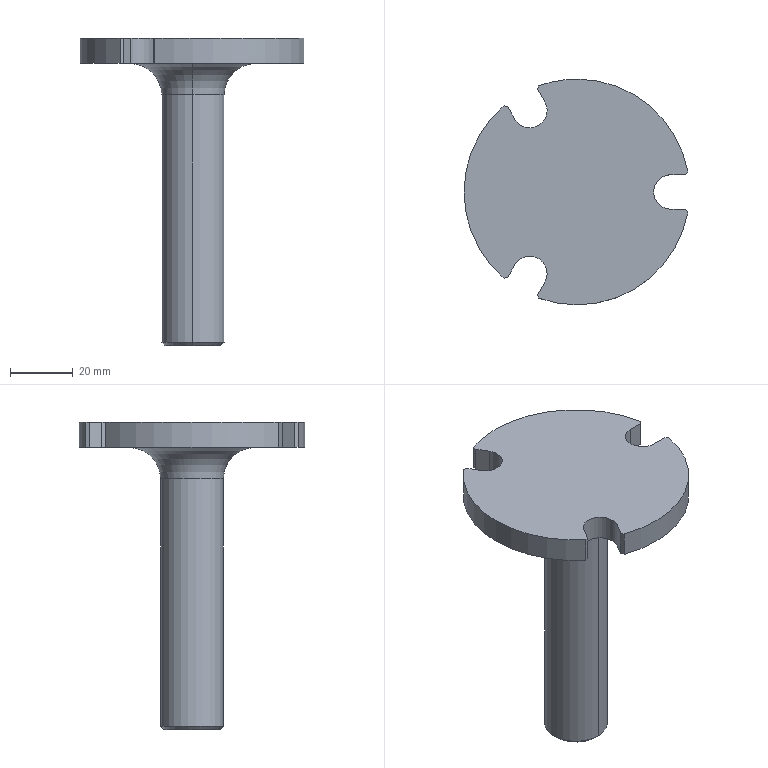Part | NX | 1 solid | 29 faces | box 71.434 x 72 x 98 mm | volume 59758 mm3 | plane 15 | cylinder 10 | torus 2 | cone 2 | commonest cylinder face diameters 11 x4 72 x4 20 x2
STEP:
#1=CARTESIAN_POINT('',(0.2829,20.,-8.));
#2=VERTEX_POINT('',#1);
#3=CARTESIAN_POINT('',(0.2829,-20.,-8.));
#4=VERTEX_POINT('',#3);
#5=CARTESIAN_POINT('',(0.2829,0.,-8.));
#6=DIRECTION('',(0.,0.,1.));
#7=DIRECTION('',(0.,-1.,0.));
#8=AXIS2_PLACEMENT_3D('',#5,#6,#7);
#9=CIRCLE('',#8,20.);
#10=EDGE_CURVE('',#2,#4,#9,.T.);
#11=ORIENTED_EDGE('',*,*,#10,.F.);
#12=CARTESIAN_POINT('',(0.2829,10.,-18.));
#13=VERTEX_POINT('',#12);
#14=CARTESIAN_POINT('',(0.2829,20.,-18.));
#15=DIRECTION('',(1.,0.,0.));
#16=DIRECTION('',(0.,1.,0.));
#17=AXIS2_PLACEMENT_3D('',#14,#15,#16);
#18=CIRCLE('',#17,10.);
#19=EDGE_CURVE('',#13,#2,#18,.F.);
#20=ORIENTED_EDGE('',*,*,#19,.F.);
#21=CARTESIAN_POINT('',(0.2829,-10.,-18.));
#22=VERTEX_POINT('',#21);
#23=CARTESIAN_POINT('',(0.2829,0.,-18.));
#24=DIRECTION('',(0.,0.,-1.));
#25=DIRECTION('',(0.,-1.,0.));
#26=AXIS2_PLACEMENT_3D('',#23,#24,#25);
#27=CIRCLE('',#26,10.);
#28=EDGE_CURVE('',#22,#13,#27,.T.);
#29=ORIENTED_EDGE('',*,*,#28,.F.);
#30=CARTESIAN_POINT('',(0.2829,-20.,-18.));
#31=DIRECTION('',(-1.,0.,0.));
#32=DIRECTION('',(0.,-1.,0.));
#33=AXIS2_PLACEMENT_3D('',#30,#31,#32);
#34=CIRCLE('',#33,10.);
#35=EDGE_CURVE('',#22,#4,#34,.F.);
#36=ORIENTED_EDGE('',*,*,#35,.T.);
#37=EDGE_LOOP('',(#11,#20,#29,#36));
#38=FACE_BOUND('',#37,.T.);
#39=CARTESIAN_POINT('',(0.2829,0.,-18.));
#40=DIRECTION('',(0.,0.,1.));
#41=DIRECTION('',(0.,1.,0.));
#42=AXIS2_PLACEMENT_3D('',#39,#40,#41);
#43=TOROIDAL_SURFACE('',#42,20.,10.);
#44=ADVANCED_FACE('',(#38),#43,.F.);
#45=CARTESIAN_POINT('',(-14.717,20.481,-8.));
#46=VERTEX_POINT('',#45);
#47=CARTESIAN_POINT('',(-9.954,28.731,-8.));
#48=VERTEX_POINT('',#47);
#49=CARTESIAN_POINT('',(-14.717,25.981,-8.));
#50=DIRECTION('',(0.,0.,1.));
#51=DIRECTION('',(0.866,0.5,0.));
#52=AXIS2_PLACEMENT_3D('',#49,#50,#51);
#53=CIRCLE('',#52,5.5);
#54=EDGE_CURVE('',#46,#48,#53,.T.);
#55=ORIENTED_EDGE('',*,*,#54,.F.);
#56=CARTESIAN_POINT('',(-14.717,20.481,0.));
#57=VERTEX_POINT('',#56);
#58=CARTESIAN_POINT('',(-14.717,20.481,-8.));
#59=DIRECTION('',(0.,0.,1.));
#60=VECTOR('',#59,1000.);
#61=LINE('',#58,#60);
#62=EDGE_CURVE('',#46,#57,#61,.T.);
#63=ORIENTED_EDGE('',*,*,#62,.T.);
#64=CARTESIAN_POINT('',(-9.954,28.731,0.));
#65=VERTEX_POINT('',#64);
#66=CARTESIAN_POINT('',(-14.717,25.981,0.));
#67=DIRECTION('',(0.,0.,1.));
#68=DIRECTION('',(0.866,0.5,0.));
#69=AXIS2_PLACEMENT_3D('',#66,#67,#68);
#70=CIRCLE('',#69,5.5);
#71=EDGE_CURVE('',#57,#65,#70,.T.);
#72=ORIENTED_EDGE('',*,*,#71,.T.);
#73=CARTESIAN_POINT('',(-9.954,28.731,-8.));
#74=DIRECTION('',(0.,0.,1.));
#75=VECTOR('',#74,1000.);
#76=LINE('',#73,#75);
#77=EDGE_CURVE('',#48,#65,#76,.T.);
#78=ORIENTED_EDGE('',*,*,#77,.F.);
#79=EDGE_LOOP('',(#55,#63,#72,#78));
#80=FACE_BOUND('',#79,.T.);
#81=CARTESIAN_POINT('',(-14.717,25.981,-8.));
#82=DIRECTION('',(0.,0.,1.));
#83=DIRECTION('',(0.,1.,0.));
#84=AXIS2_PLACEMENT_3D('',#81,#82,#83);
#85=CYLINDRICAL_SURFACE('',#84,5.5);
#86=ADVANCED_FACE('',(#80),#85,.F.);
#87=CARTESIAN_POINT('',(0.2829,36.,0.));
#88=VERTEX_POINT('',#87);
#89=CARTESIAN_POINT('',(-11.929,33.865,0.));
#90=VERTEX_POINT('',#89);
#91=CARTESIAN_POINT('',(0.2829,0.,0.));
#92=DIRECTION('',(0.,0.,1.));
#93=DIRECTION('',(0.,-1.,0.));
#94=AXIS2_PLACEMENT_3D('',#91,#92,#93);
#95=CIRCLE('',#94,36.);
#96=EDGE_CURVE('',#88,#90,#95,.T.);
#97=ORIENTED_EDGE('',*,*,#96,.F.);
#98=CARTESIAN_POINT('',(0.2829,36.,-8.));
#99=VERTEX_POINT('',#98);
#100=CARTESIAN_POINT('',(0.2829,36.,0.));
#101=DIRECTION('',(0.,0.,-1.));
#102=VECTOR('',#101,1000.);
#103=LINE('',#100,#102);
#104=EDGE_CURVE('',#88,#99,#103,.T.);
#105=ORIENTED_EDGE('',*,*,#104,.T.);
#106=CARTESIAN_POINT('',(-11.929,33.865,-8.));
#107=VERTEX_POINT('',#106);
#108=CARTESIAN_POINT('',(0.2829,0.,-8.));
#109=DIRECTION('',(0.,0.,1.));
#110=DIRECTION('',(0.,-1.,0.));
#111=AXIS2_PLACEMENT_3D('',#108,#109,#110);
#112=CIRCLE('',#111,36.);
#113=EDGE_CURVE('',#99,#107,#112,.T.);
#114=ORIENTED_EDGE('',*,*,#113,.T.);
#115=CARTESIAN_POINT('',(-11.929,33.865,0.));
#116=DIRECTION('',(0.,0.,1.));
#117=VECTOR('',#116,1000.);
#118=LINE('',#115,#117);
#119=EDGE_CURVE('',#107,#90,#118,.T.);
#120=ORIENTED_EDGE('',*,*,#119,.T.);
#121=EDGE_LOOP('',(#97,#105,#114,#120));
#122=FACE_BOUND('',#121,.T.);
#123=CARTESIAN_POINT('',(0.2829,0.,0.));
#124=DIRECTION('',(0.,0.,-1.));
#125=DIRECTION('',(0.,-1.,0.));
#126=AXIS2_PLACEMENT_3D('',#123,#124,#125);
#127=CYLINDRICAL_SURFACE('',#126,36.);
#128=ADVANCED_FACE('',(#122),#127,.T.);
#129=CARTESIAN_POINT('',(0.2829,9.,-98.));
#130=VERTEX_POINT('',#129);
#131=CARTESIAN_POINT('',(0.2829,-9.,-98.));
#132=VERTEX_POINT('',#131);
#133=CARTESIAN_POINT('',(0.2829,0.,-98.));
#134=DIRECTION('',(0.,0.,-1.));
#135=DIRECTION('',(0.,-1.,0.));
#136=AXIS2_PLACEMENT_3D('',#133,#134,#135);
#137=CIRCLE('',#136,9.);
#138=EDGE_CURVE('',#130,#132,#137,.T.);
#139=ORIENTED_EDGE('',*,*,#138,.F.);
#140=CARTESIAN_POINT('',(0.2829,10.,-97.));
#141=VERTEX_POINT('',#140);
#142=CARTESIAN_POINT('',(0.2829,10.,-97.));
#143=DIRECTION('',(0.,0.7071,0.7071));
#144=VECTOR('',#143,1000.);
#145=LINE('',#142,#144);
#146=EDGE_CURVE('',#141,#130,#145,.F.);
#147=ORIENTED_EDGE('',*,*,#146,.F.);
#148=CARTESIAN_POINT('',(0.2829,-10.,-97.));
#149=VERTEX_POINT('',#148);
#150=CARTESIAN_POINT('',(0.2829,0.,-97.));
#151=DIRECTION('',(0.,0.,1.));
#152=DIRECTION('',(0.,-1.,0.));
#153=AXIS2_PLACEMENT_3D('',#150,#151,#152);
#154=CIRCLE('',#153,10.);
#155=EDGE_CURVE('',#149,#141,#154,.T.);
#156=ORIENTED_EDGE('',*,*,#155,.F.);
#157=CARTESIAN_POINT('',(0.2829,-10.,-97.));
#158=DIRECTION('',(0.,-0.7071,0.7071));
#159=VECTOR('',#158,1000.);
#160=LINE('',#157,#159);
#161=EDGE_CURVE('',#149,#132,#160,.F.);
#162=ORIENTED_EDGE('',*,*,#161,.T.);
#163=EDGE_LOOP('',(#139,#147,#156,#162));
#164=FACE_BOUND('',#163,.T.);
#165=CARTESIAN_POINT('',(0.2829,0.,-97.));
#166=DIRECTION('',(0.,0.,1.));
#167=DIRECTION('',(0.,1.,0.));
#168=AXIS2_PLACEMENT_3D('',#165,#166,#167);
#169=CONICAL_SURFACE('',#168,10.,0.7854);
#170=ADVANCED_FACE('',(#164),#169,.T.);
#171=CARTESIAN_POINT('',(0.2829,0.,-18.));
#172=DIRECTION('',(0.,0.,-1.));
#173=DIRECTION('',(0.,-1.,0.));
#174=AXIS2_PLACEMENT_3D('',#171,#172,#173);
#175=CIRCLE('',#174,10.);
#176=EDGE_CURVE('',#13,#22,#175,.T.);
#177=ORIENTED_EDGE('',*,*,#176,.T.);
#178=CARTESIAN_POINT('',(0.2829,-10.,-8.));
#179=DIRECTION('',(0.,0.,-1.));
#180=VECTOR('',#179,1000.);
#181=LINE('',#178,#180);
#182=EDGE_CURVE('',#149,#22,#181,.F.);
#183=ORIENTED_EDGE('',*,*,#182,.F.);
#184=ORIENTED_EDGE('',*,*,#155,.T.);
#185=CARTESIAN_POINT('',(0.2829,10.,-8.));
#186=DIRECTION('',(0.,0.,-1.));
#187=VECTOR('',#186,1000.);
#188=LINE('',#185,#187);
#189=EDGE_CURVE('',#141,#13,#188,.F.);
#190=ORIENTED_EDGE('',*,*,#189,.T.);
#191=EDGE_LOOP('',(#177,#183,#184,#190));
#192=FACE_BOUND('',#191,.T.);
#193=CARTESIAN_POINT('',(0.2829,0.,-8.));
#194=DIRECTION('',(0.,0.,-1.));
#195=DIRECTION('',(0.,-1.,0.));
#196=AXIS2_PLACEMENT_3D('',#193,#194,#195);
#197=CYLINDRICAL_SURFACE('',#196,10.);
#198=ADVANCED_FACE('',(#192),#197,.T.);
#199=CARTESIAN_POINT('',(-11.929,-33.865,0.));
#200=VERTEX_POINT('',#199);
#201=CARTESIAN_POINT('',(35.717,-6.357,0.));
#202=VERTEX_POINT('',#201);
#203=CARTESIAN_POINT('',(0.2829,0.,0.));
#204=DIRECTION('',(0.,0.,1.));
#205=DIRECTION('',(0.,-1.,0.));
#206=AXIS2_PLACEMENT_3D('',#203,#204,#205);
#207=CIRCLE('',#206,36.);
#208=EDGE_CURVE('',#200,#202,#207,.T.);
#209=ORIENTED_EDGE('',*,*,#208,.F.);
#210=CARTESIAN_POINT('',(-11.929,-33.865,-8.));
#211=VERTEX_POINT('',#210);
#212=CARTESIAN_POINT('',(-11.929,-33.865,0.));
#213=DIRECTION('',(0.,0.,-1.));
#214=VECTOR('',#213,1000.);
#215=LINE('',#212,#214);
#216=EDGE_CURVE('',#200,#211,#215,.T.);
#217=ORIENTED_EDGE('',*,*,#216,.T.);
#218=CARTESIAN_POINT('',(35.717,-6.357,-8.));
#219=VERTEX_POINT('',#218);
#220=CARTESIAN_POINT('',(0.2829,0.,-8.));
#221=DIRECTION('',(0.,0.,1.));
#222=DIRECTION('',(0.,-1.,0.));
#223=AXIS2_PLACEMENT_3D('',#220,#221,#222);
#224=CIRCLE('',#223,36.);
#225=EDGE_CURVE('',#211,#219,#224,.T.);
#226=ORIENTED_EDGE('',*,*,#225,.T.);
#227=CARTESIAN_POINT('',(35.717,-6.357,0.));
#228=DIRECTION('',(0.,0.,1.));
#229=VECTOR('',#228,1000.);
#230=LINE('',#227,#229);
#231=EDGE_CURVE('',#219,#202,#230,.T.);
#232=ORIENTED_EDGE('',*,*,#231,.T.);
#233=EDGE_LOOP('',(#209,#217,#226,#232));
#234=FACE_BOUND('',#233,.T.);
#235=CARTESIAN_POINT('',(0.2829,0.,0.));
#236=DIRECTION('',(0.,0.,-1.));
#237=DIRECTION('',(0.,-1.,0.));
#238=AXIS2_PLACEMENT_3D('',#235,#236,#237);
#239=CYLINDRICAL_SURFACE('',#238,36.);
#240=ADVANCED_FACE('',(#234),#239,.T.);
#241=CARTESIAN_POINT('',(-22.94,27.509,0.));
#242=VERTEX_POINT('',#241);
#243=CARTESIAN_POINT('',(-22.94,-27.509,0.));
#244=VERTEX_POINT('',#243);
#245=CARTESIAN_POINT('',(0.2829,0.,0.));
#246=DIRECTION('',(0.,0.,1.));
#247=DIRECTION('',(0.,-1.,0.));
#248=AXIS2_PLACEMENT_3D('',#245,#246,#247);
#249=CIRCLE('',#248,36.);
#250=EDGE_CURVE('',#242,#244,#249,.T.);
#251=ORIENTED_EDGE('',*,*,#250,.F.);
#252=CARTESIAN_POINT('',(-22.94,27.509,-8.));
#253=VERTEX_POINT('',#252);
#254=CARTESIAN_POINT('',(-22.94,27.509,0.));
#255=DIRECTION('',(0.,0.,-1.));
#256=VECTOR('',#255,1000.);
#257=LINE('',#254,#256);
#258=EDGE_CURVE('',#242,#253,#257,.T.);
#259=ORIENTED_EDGE('',*,*,#258,.T.);
#260=CARTESIAN_POINT('',(-22.94,-27.509,-8.));
#261=VERTEX_POINT('',#260);
#262=CARTESIAN_POINT('',(0.2829,0.,-8.));
#263=DIRECTION('',(0.,0.,1.));
#264=DIRECTION('',(0.,-1.,0.));
#265=AXIS2_PLACEMENT_3D('',#262,#263,#264);
#266=CIRCLE('',#265,36.);
#267=EDGE_CURVE('',#253,#261,#266,.T.);
#268=ORIENTED_EDGE('',*,*,#267,.T.);
#269=CARTESIAN_POINT('',(-22.94,-27.509,0.));
#270=DIRECTION('',(0.,0.,1.));
#271=VECTOR('',#270,1000.);
#272=LINE('',#269,#271);
#273=EDGE_CURVE('',#261,#244,#272,.T.);
#274=ORIENTED_EDGE('',*,*,#273,.T.);
#275=EDGE_LOOP('',(#251,#259,#268,#274));
#276=FACE_BOUND('',#275,.T.);
#277=CARTESIAN_POINT('',(0.2829,0.,0.));
#278=DIRECTION('',(0.,0.,-1.));
#279=DIRECTION('',(0.,-1.,0.));
#280=AXIS2_PLACEMENT_3D('',#277,#278,#279);
#281=CYLINDRICAL_SURFACE('',#280,36.);
#282=ADVANCED_FACE('',(#276),#281,.T.);
#283=ORIENTED_EDGE('',*,*,#182,.T.);
#284=ORIENTED_EDGE('',*,*,#28,.T.);
#285=ORIENTED_EDGE('',*,*,#189,.F.);
#286=CARTESIAN_POINT('',(0.2829,0.,-97.));
#287=DIRECTION('',(0.,0.,1.));
#288=DIRECTION('',(0.,-1.,0.));
#289=AXIS2_PLACEMENT_3D('',#286,#287,#288);
#290=CIRCLE('',#289,10.);
#291=EDGE_CURVE('',#141,#149,#290,.T.);
#292=ORIENTED_EDGE('',*,*,#291,.T.);
#293=EDGE_LOOP('',(#283,#284,#285,#292));
#294=FACE_BOUND('',#293,.T.);
#295=CARTESIAN_POINT('',(0.2829,0.,-8.));
#296=DIRECTION('',(0.,0.,-1.));
#297=DIRECTION('',(0.,-1.,0.));
#298=AXIS2_PLACEMENT_3D('',#295,#296,#297);
#299=CYLINDRICAL_SURFACE('',#298,10.);
#300=ADVANCED_FACE('',(#294),#299,.T.);
#301=CARTESIAN_POINT('',(0.2829,0.,-98.));
#302=DIRECTION('',(0.,0.,-1.));
#303=DIRECTION('',(0.,-1.,0.));
#304=AXIS2_PLACEMENT_3D('',#301,#302,#303);
#305=CIRCLE('',#304,9.);
#306=EDGE_CURVE('',#132,#130,#305,.T.);
#307=ORIENTED_EDGE('',*,*,#306,.T.);
#308=ORIENTED_EDGE('',*,*,#138,.T.);
#309=EDGE_LOOP('',(#307,#308));
#310=FACE_BOUND('',#309,.T.);
#311=CARTESIAN_POINT('',(0.2829,0.,-98.));
#312=DIRECTION('',(0.,0.,1.));
#313=DIRECTION('',(0.,1.,0.));
#314=AXIS2_PLACEMENT_3D('',#311,#312,#313);
#315=PLANE('',#314);
#316=ADVANCED_FACE('',(#310),#315,.F.);
#317=ORIENTED_EDGE('',*,*,#146,.T.);
#318=ORIENTED_EDGE('',*,*,#306,.F.);
#319=ORIENTED_EDGE('',*,*,#161,.F.);
#320=ORIENTED_EDGE('',*,*,#291,.F.);
#321=EDGE_LOOP('',(#317,#318,#319,#320));
#322=FACE_BOUND('',#321,.T.);
#323=CARTESIAN_POINT('',(0.2829,0.,-97.));
#324=DIRECTION('',(0.,0.,1.));
#325=DIRECTION('',(0.,1.,0.));
#326=AXIS2_PLACEMENT_3D('',#323,#324,#325);
#327=CONICAL_SURFACE('',#326,10.,0.7854);
#328=ADVANCED_FACE('',(#322),#327,.T.);
#329=ORIENTED_EDGE('',*,*,#104,.F.);
#330=CARTESIAN_POINT('',(35.717,6.357,0.));
#331=VERTEX_POINT('',#330);
#332=CARTESIAN_POINT('',(0.2829,0.,0.));
#333=DIRECTION('',(0.,0.,1.));
#334=DIRECTION('',(0.,-1.,0.));
#335=AXIS2_PLACEMENT_3D('',#332,#333,#334);
#336=CIRCLE('',#335,36.);
#337=EDGE_CURVE('',#331,#88,#336,.T.);
#338=ORIENTED_EDGE('',*,*,#337,.F.);
#339=CARTESIAN_POINT('',(35.717,6.357,-8.));
#340=VERTEX_POINT('',#339);
#341=CARTESIAN_POINT('',(35.717,6.357,0.));
#342=DIRECTION('',(0.,0.,-1.));
#343=VECTOR('',#342,1000.);
#344=LINE('',#341,#343);
#345=EDGE_CURVE('',#331,#340,#344,.T.);
#346=ORIENTED_EDGE('',*,*,#345,.T.);
#347=CARTESIAN_POINT('',(0.2829,0.,-8.));
#348=DIRECTION('',(0.,0.,1.));
#349=DIRECTION('',(0.,-1.,0.));
#350=AXIS2_PLACEMENT_3D('',#347,#348,#349);
#351=CIRCLE('',#350,36.);
#352=EDGE_CURVE('',#340,#99,#351,.T.);
#353=ORIENTED_EDGE('',*,*,#352,.T.);
#354=EDGE_LOOP('',(#329,#338,#346,#353));
#355=FACE_BOUND('',#354,.T.);
#356=CARTESIAN_POINT('',(0.2829,0.,0.));
#357=DIRECTION('',(0.,0.,-1.));
#358=DIRECTION('',(0.,-1.,0.));
#359=AXIS2_PLACEMENT_3D('',#356,#357,#358);
#360=CYLINDRICAL_SURFACE('',#359,36.);
#361=ADVANCED_FACE('',(#355),#360,.T.);
#362=ORIENTED_EDGE('',*,*,#337,.T.);
#363=ORIENTED_EDGE('',*,*,#96,.T.);
#364=CARTESIAN_POINT('',(-12.243,32.695,0.));
#365=VERTEX_POINT('',#364);
#366=CARTESIAN_POINT('',(-19.577,5.322,0.));
#367=DIRECTION('',(-0.2588,-0.9659,0.));
#368=VECTOR('',#367,1000.);
#369=LINE('',#366,#368);
#370=EDGE_CURVE('',#90,#365,#369,.T.);
#371=ORIENTED_EDGE('',*,*,#370,.T.);
#372=CARTESIAN_POINT('',(-9.954,28.731,0.));
#373=DIRECTION('',(-0.5,0.866,0.));
#374=VECTOR('',#373,1000.);
#375=LINE('',#372,#374);
#376=EDGE_CURVE('',#65,#365,#375,.T.);
#377=ORIENTED_EDGE('',*,*,#376,.F.);
#378=ORIENTED_EDGE('',*,*,#71,.F.);
#379=CARTESIAN_POINT('',(-19.48,23.231,0.));
#380=VERTEX_POINT('',#379);
#381=CARTESIAN_POINT('',(-14.717,25.981,0.));
#382=DIRECTION('',(0.,0.,1.));
#383=DIRECTION('',(0.866,0.5,0.));
#384=AXIS2_PLACEMENT_3D('',#381,#382,#383);
#385=CIRCLE('',#384,5.5);
#386=EDGE_CURVE('',#380,#57,#385,.T.);
#387=ORIENTED_EDGE('',*,*,#386,.F.);
#388=CARTESIAN_POINT('',(-21.769,27.195,0.));
#389=VERTEX_POINT('',#388);
#390=CARTESIAN_POINT('',(-19.48,23.231,0.));
#391=DIRECTION('',(0.5,-0.866,0.));
#392=VECTOR('',#391,1000.);
#393=LINE('',#390,#392);
#394=EDGE_CURVE('',#389,#380,#393,.T.);
#395=ORIENTED_EDGE('',*,*,#394,.F.);
#396=CARTESIAN_POINT('',(5.604,19.86,0.));
#397=DIRECTION('',(-0.9659,0.2588,0.));
#398=VECTOR('',#397,1000.);
#399=LINE('',#396,#398);
#400=EDGE_CURVE('',#389,#242,#399,.T.);
#401=ORIENTED_EDGE('',*,*,#400,.T.);
#402=ORIENTED_EDGE('',*,*,#250,.T.);
#403=CARTESIAN_POINT('',(-21.769,-27.195,0.));
#404=VERTEX_POINT('',#403);
#405=CARTESIAN_POINT('',(5.604,-19.86,0.));
#406=DIRECTION('',(0.9659,0.2588,0.));
#407=VECTOR('',#406,1000.);
#408=LINE('',#405,#407);
#409=EDGE_CURVE('',#244,#404,#408,.T.);
#410=ORIENTED_EDGE('',*,*,#409,.T.);
#411=CARTESIAN_POINT('',(-19.48,-23.231,0.));
#412=VERTEX_POINT('',#411);
#413=CARTESIAN_POINT('',(-19.48,-23.231,0.));
#414=DIRECTION('',(-0.5,-0.866,0.));
#415=VECTOR('',#414,1000.);
#416=LINE('',#413,#415);
#417=EDGE_CURVE('',#412,#404,#416,.T.);
#418=ORIENTED_EDGE('',*,*,#417,.F.);
#419=CARTESIAN_POINT('',(-9.954,-28.731,0.));
#420=VERTEX_POINT('',#419);
#421=CARTESIAN_POINT('',(-14.717,-25.981,0.));
#422=DIRECTION('',(0.,0.,1.));
#423=DIRECTION('',(-0.866,0.5,0.));
#424=AXIS2_PLACEMENT_3D('',#421,#422,#423);
#425=CIRCLE('',#424,5.5);
#426=EDGE_CURVE('',#420,#412,#425,.T.);
#427=ORIENTED_EDGE('',*,*,#426,.F.);
#428=CARTESIAN_POINT('',(-12.243,-32.695,0.));
#429=VERTEX_POINT('',#428);
#430=CARTESIAN_POINT('',(-9.954,-28.731,0.));
#431=DIRECTION('',(0.5,0.866,0.));
#432=VECTOR('',#431,1000.);
#433=LINE('',#430,#432);
#434=EDGE_CURVE('',#429,#420,#433,.T.);
#435=ORIENTED_EDGE('',*,*,#434,.F.);
#436=CARTESIAN_POINT('',(-19.577,-5.322,0.));
#437=DIRECTION('',(0.2588,-0.9659,0.));
#438=VECTOR('',#437,1000.);
#439=LINE('',#436,#438);
#440=EDGE_CURVE('',#429,#200,#439,.T.);
#441=ORIENTED_EDGE('',*,*,#440,.T.);
#442=ORIENTED_EDGE('',*,*,#208,.T.);
#443=CARTESIAN_POINT('',(34.86,-5.5,0.));
#444=VERTEX_POINT('',#443);
#445=CARTESIAN_POINT('',(14.822,14.539,0.));
#446=DIRECTION('',(-0.7071,0.7071,0.));
#447=VECTOR('',#446,1000.);
#448=LINE('',#445,#447);
#449=EDGE_CURVE('',#202,#444,#448,.T.);
#450=ORIENTED_EDGE('',*,*,#449,.T.);
#451=CARTESIAN_POINT('',(30.283,-5.5,0.));
#452=VERTEX_POINT('',#451);
#453=CARTESIAN_POINT('',(30.283,-5.5,0.));
#454=DIRECTION('',(1.,0.,0.));
#455=VECTOR('',#454,1000.);
#456=LINE('',#453,#455);
#457=EDGE_CURVE('',#452,#444,#456,.T.);
#458=ORIENTED_EDGE('',*,*,#457,.F.);
#459=CARTESIAN_POINT('',(30.283,5.5,0.));
#460=VERTEX_POINT('',#459);
#461=CARTESIAN_POINT('',(30.283,0.,0.));
#462=DIRECTION('',(0.,0.,1.));
#463=DIRECTION('',(0.,-1.,0.));
#464=AXIS2_PLACEMENT_3D('',#461,#462,#463);
#465=CIRCLE('',#464,5.5);
#466=EDGE_CURVE('',#460,#452,#465,.T.);
#467=ORIENTED_EDGE('',*,*,#466,.F.);
#468=CARTESIAN_POINT('',(34.86,5.5,0.));
#469=VERTEX_POINT('',#468);
#470=CARTESIAN_POINT('',(30.283,5.5,0.));
#471=DIRECTION('',(-1.,0.,0.));
#472=VECTOR('',#471,1000.);
#473=LINE('',#470,#472);
#474=EDGE_CURVE('',#469,#460,#473,.T.);
#475=ORIENTED_EDGE('',*,*,#474,.F.);
#476=CARTESIAN_POINT('',(14.822,-14.539,0.));
#477=DIRECTION('',(0.7071,0.7071,0.));
#478=VECTOR('',#477,1000.);
#479=LINE('',#476,#478);
#480=EDGE_CURVE('',#469,#331,#479,.T.);
#481=ORIENTED_EDGE('',*,*,#480,.T.);
#482=EDGE_LOOP('',(#362,#363,#371,#377,#378,#387,#395,#401,#402,#410,#418,#427,#435,#441,#442,#450,#458,#467,#475,#481));
#483=FACE_BOUND('',#482,.T.);
#484=CARTESIAN_POINT('',(0.2829,0.,0.));
#485=DIRECTION('',(0.,0.,1.));
#486=DIRECTION('',(0.,1.,0.));
#487=AXIS2_PLACEMENT_3D('',#484,#485,#486);
#488=PLANE('',#487);
#489=ADVANCED_FACE('',(#483),#488,.T.);
#490=CARTESIAN_POINT('',(0.2829,0.,-8.));
#491=DIRECTION('',(0.,0.,1.));
#492=DIRECTION('',(0.,-1.,0.));
#493=AXIS2_PLACEMENT_3D('',#490,#491,#492);
#494=CIRCLE('',#493,20.);
#495=EDGE_CURVE('',#4,#2,#494,.T.);
#496=ORIENTED_EDGE('',*,*,#495,.T.);
#497=ORIENTED_EDGE('',*,*,#10,.T.);
#498=EDGE_LOOP('',(#496,#497));
#499=FACE_BOUND('',#498,.T.);
#500=CARTESIAN_POINT('',(-12.243,32.695,-8.));
#501=VERTEX_POINT('',#500);
#502=CARTESIAN_POINT('',(-9.954,28.731,-8.));
#503=DIRECTION('',(-0.5,0.866,0.));
#504=VECTOR('',#503,1000.);
#505=LINE('',#502,#504);
#506=EDGE_CURVE('',#48,#501,#505,.T.);
#507=ORIENTED_EDGE('',*,*,#506,.T.);
#508=CARTESIAN_POINT('',(-11.929,33.865,-8.));
#509=DIRECTION('',(0.2588,0.9659,0.));
#510=VECTOR('',#509,1000.);
#511=LINE('',#508,#510);
#512=EDGE_CURVE('',#501,#107,#511,.T.);
#513=ORIENTED_EDGE('',*,*,#512,.T.);
#514=ORIENTED_EDGE('',*,*,#113,.F.);
#515=ORIENTED_EDGE('',*,*,#352,.F.);
#516=CARTESIAN_POINT('',(34.86,5.5,-8.));
#517=VERTEX_POINT('',#516);
#518=CARTESIAN_POINT('',(35.717,6.357,-8.));
#519=DIRECTION('',(-0.7071,-0.7071,0.));
#520=VECTOR('',#519,1000.);
#521=LINE('',#518,#520);
#522=EDGE_CURVE('',#340,#517,#521,.T.);
#523=ORIENTED_EDGE('',*,*,#522,.T.);
#524=CARTESIAN_POINT('',(30.283,5.5,-8.));
#525=VERTEX_POINT('',#524);
#526=CARTESIAN_POINT('',(0.2829,5.5,-8.));
#527=DIRECTION('',(-1.,0.,0.));
#528=VECTOR('',#527,1000.);
#529=LINE('',#526,#528);
#530=EDGE_CURVE('',#517,#525,#529,.T.);
#531=ORIENTED_EDGE('',*,*,#530,.T.);
#532=CARTESIAN_POINT('',(30.283,-5.5,-8.));
#533=VERTEX_POINT('',#532);
#534=CARTESIAN_POINT('',(30.283,0.,-8.));
#535=DIRECTION('',(0.,0.,1.));
#536=DIRECTION('',(0.,-1.,0.));
#537=AXIS2_PLACEMENT_3D('',#534,#535,#536);
#538=CIRCLE('',#537,5.5);
#539=EDGE_CURVE('',#525,#533,#538,.T.);
#540=ORIENTED_EDGE('',*,*,#539,.T.);
#541=CARTESIAN_POINT('',(34.86,-5.5,-8.));
#542=VERTEX_POINT('',#541);
#543=CARTESIAN_POINT('',(30.283,-5.5,-8.));
#544=DIRECTION('',(1.,0.,0.));
#545=VECTOR('',#544,1000.);
#546=LINE('',#543,#545);
#547=EDGE_CURVE('',#533,#542,#546,.T.);
#548=ORIENTED_EDGE('',*,*,#547,.T.);
#549=CARTESIAN_POINT('',(35.717,-6.357,-8.));
#550=DIRECTION('',(0.7071,-0.7071,0.));
#551=VECTOR('',#550,1000.);
#552=LINE('',#549,#551);
#553=EDGE_CURVE('',#542,#219,#552,.T.);
#554=ORIENTED_EDGE('',*,*,#553,.T.);
#555=ORIENTED_EDGE('',*,*,#225,.F.);
#556=CARTESIAN_POINT('',(-12.243,-32.695,-8.));
#557=VERTEX_POINT('',#556);
#558=CARTESIAN_POINT('',(-11.929,-33.865,-8.));
#559=DIRECTION('',(-0.2588,0.9659,0.));
#560=VECTOR('',#559,1000.);
#561=LINE('',#558,#560);
#562=EDGE_CURVE('',#211,#557,#561,.T.);
#563=ORIENTED_EDGE('',*,*,#562,.T.);
#564=CARTESIAN_POINT('',(-9.954,-28.731,-8.));
#565=VERTEX_POINT('',#564);
#566=CARTESIAN_POINT('',(5.046,-2.75,-8.));
#567=DIRECTION('',(0.5,0.866,0.));
#568=VECTOR('',#567,1000.);
#569=LINE('',#566,#568);
#570=EDGE_CURVE('',#557,#565,#569,.T.);
#571=ORIENTED_EDGE('',*,*,#570,.T.);
#572=CARTESIAN_POINT('',(-19.48,-23.231,-8.));
#573=VERTEX_POINT('',#572);
#574=CARTESIAN_POINT('',(-14.717,-25.981,-8.));
#575=DIRECTION('',(0.,0.,1.));
#576=DIRECTION('',(-0.866,0.5,0.));
#577=AXIS2_PLACEMENT_3D('',#574,#575,#576);
#578=CIRCLE('',#577,5.5);
#579=EDGE_CURVE('',#565,#573,#578,.T.);
#580=ORIENTED_EDGE('',*,*,#579,.T.);
#581=CARTESIAN_POINT('',(-21.769,-27.195,-8.));
#582=VERTEX_POINT('',#581);
#583=CARTESIAN_POINT('',(-19.48,-23.231,-8.));
#584=DIRECTION('',(-0.5,-0.866,0.));
#585=VECTOR('',#584,1000.);
#586=LINE('',#583,#585);
#587=EDGE_CURVE('',#573,#582,#586,.T.);
#588=ORIENTED_EDGE('',*,*,#587,.T.);
#589=CARTESIAN_POINT('',(-22.94,-27.509,-8.));
#590=DIRECTION('',(-0.9659,-0.2588,0.));
#591=VECTOR('',#590,1000.);
#592=LINE('',#589,#591);
#593=EDGE_CURVE('',#582,#261,#592,.T.);
#594=ORIENTED_EDGE('',*,*,#593,.T.);
#595=ORIENTED_EDGE('',*,*,#267,.F.);
#596=CARTESIAN_POINT('',(-21.769,27.195,-8.));
#597=VERTEX_POINT('',#596);
#598=CARTESIAN_POINT('',(-22.94,27.509,-8.));
#599=DIRECTION('',(0.9659,-0.2588,0.));
#600=VECTOR('',#599,1000.);
#601=LINE('',#598,#600);
#602=EDGE_CURVE('',#253,#597,#601,.T.);
#603=ORIENTED_EDGE('',*,*,#602,.T.);
#604=CARTESIAN_POINT('',(-19.48,23.231,-8.));
#605=VERTEX_POINT('',#604);
#606=CARTESIAN_POINT('',(-4.48,-2.75,-8.));
#607=DIRECTION('',(0.5,-0.866,0.));
#608=VECTOR('',#607,1000.);
#609=LINE('',#606,#608);
#610=EDGE_CURVE('',#597,#605,#609,.T.);
#611=ORIENTED_EDGE('',*,*,#610,.T.);
#612=CARTESIAN_POINT('',(-14.717,25.981,-8.));
#613=DIRECTION('',(0.,0.,1.));
#614=DIRECTION('',(0.866,0.5,0.));
#615=AXIS2_PLACEMENT_3D('',#612,#613,#614);
#616=CIRCLE('',#615,5.5);
#617=EDGE_CURVE('',#605,#46,#616,.T.);
#618=ORIENTED_EDGE('',*,*,#617,.T.);
#619=ORIENTED_EDGE('',*,*,#54,.T.);
#620=EDGE_LOOP('',(#507,#513,#514,#515,#523,#531,#540,#548,#554,#555,#563,#571,#580,#588,#594,#595,#603,#611,#618,#619));
#621=FACE_BOUND('',#620,.T.);
#622=CARTESIAN_POINT('',(0.2829,0.,-8.));
#623=DIRECTION('',(0.,0.,1.));
#624=DIRECTION('',(0.,1.,0.));
#625=AXIS2_PLACEMENT_3D('',#622,#623,#624);
#626=PLANE('',#625);
#627=ADVANCED_FACE('',(#499,#621),#626,.F.);
#628=ORIENTED_EDGE('',*,*,#530,.F.);
#629=CARTESIAN_POINT('',(34.86,5.5,-8.));
#630=DIRECTION('',(0.,0.,1.));
#631=VECTOR('',#630,1000.);
#632=LINE('',#629,#631);
#633=EDGE_CURVE('',#517,#469,#632,.T.);
#634=ORIENTED_EDGE('',*,*,#633,.T.);
#635=ORIENTED_EDGE('',*,*,#474,.T.);
#636=CARTESIAN_POINT('',(30.283,5.5,-8.));
#637=DIRECTION('',(0.,0.,1.));
#638=VECTOR('',#637,1000.);
#639=LINE('',#636,#638);
#640=EDGE_CURVE('',#525,#460,#639,.T.);
#641=ORIENTED_EDGE('',*,*,#640,.F.);
#642=EDGE_LOOP('',(#628,#634,#635,#641));
#643=FACE_BOUND('',#642,.T.);
#644=CARTESIAN_POINT('',(30.283,5.5,-8.));
#645=DIRECTION('',(0.,1.,0.));
#646=DIRECTION('',(1.,0.,0.));
#647=AXIS2_PLACEMENT_3D('',#644,#645,#646);
#648=PLANE('',#647);
#649=ADVANCED_FACE('',(#643),#648,.F.);
#650=ORIENTED_EDGE('',*,*,#457,.T.);
#651=CARTESIAN_POINT('',(34.86,-5.5,-8.));
#652=DIRECTION('',(0.,0.,-1.));
#653=VECTOR('',#652,1000.);
#654=LINE('',#651,#653);
#655=EDGE_CURVE('',#444,#542,#654,.T.);
#656=ORIENTED_EDGE('',*,*,#655,.T.);
#657=ORIENTED_EDGE('',*,*,#547,.F.);
#658=CARTESIAN_POINT('',(30.283,-5.5,-8.));
#659=DIRECTION('',(0.,0.,1.));
#660=VECTOR('',#659,1000.);
#661=LINE('',#658,#660);
#662=EDGE_CURVE('',#533,#452,#661,.T.);
#663=ORIENTED_EDGE('',*,*,#662,.T.);
#664=EDGE_LOOP('',(#650,#656,#657,#663));
#665=FACE_BOUND('',#664,.T.);
#666=CARTESIAN_POINT('',(30.283,-5.5,-8.));
#667=DIRECTION('',(0.,-1.,0.));
#668=DIRECTION('',(-1.,0.,0.));
#669=AXIS2_PLACEMENT_3D('',#666,#667,#668);
#670=PLANE('',#669);
#671=ADVANCED_FACE('',(#665),#670,.F.);
#672=ORIENTED_EDGE('',*,*,#466,.T.);
#673=ORIENTED_EDGE('',*,*,#662,.F.);
#674=ORIENTED_EDGE('',*,*,#539,.F.);
#675=ORIENTED_EDGE('',*,*,#640,.T.);
#676=EDGE_LOOP('',(#672,#673,#674,#675));
#677=FACE_BOUND('',#676,.T.);
#678=CARTESIAN_POINT('',(30.283,0.,-8.));
#679=DIRECTION('',(0.,0.,1.));
#680=DIRECTION('',(0.,1.,0.));
#681=AXIS2_PLACEMENT_3D('',#678,#679,#680);
#682=CYLINDRICAL_SURFACE('',#681,5.5);
#683=ADVANCED_FACE('',(#677),#682,.F.);
#684=ORIENTED_EDGE('',*,*,#610,.F.);
#685=CARTESIAN_POINT('',(-21.769,27.195,-8.));
#686=DIRECTION('',(0.,0.,1.));
#687=VECTOR('',#686,1000.);
#688=LINE('',#685,#687);
#689=EDGE_CURVE('',#597,#389,#688,.T.);
#690=ORIENTED_EDGE('',*,*,#689,.T.);
#691=ORIENTED_EDGE('',*,*,#394,.T.);
#692=CARTESIAN_POINT('',(-19.48,23.231,-8.));
#693=DIRECTION('',(0.,0.,1.));
#694=VECTOR('',#693,1000.);
#695=LINE('',#692,#694);
#696=EDGE_CURVE('',#605,#380,#695,.T.);
#697=ORIENTED_EDGE('',*,*,#696,.F.);
#698=EDGE_LOOP('',(#684,#690,#691,#697));
#699=FACE_BOUND('',#698,.T.);
#700=CARTESIAN_POINT('',(-19.48,23.231,-8.));
#701=DIRECTION('',(-0.866,-0.5,0.));
#702=DIRECTION('',(-0.5,0.866,0.));
#703=AXIS2_PLACEMENT_3D('',#700,#701,#702);
#704=PLANE('',#703);
#705=ADVANCED_FACE('',(#699),#704,.F.);
#706=ORIENTED_EDGE('',*,*,#376,.T.);
#707=CARTESIAN_POINT('',(-12.243,32.695,-8.));
#708=DIRECTION('',(0.,0.,-1.));
#709=VECTOR('',#708,1000.);
#710=LINE('',#707,#709);
#711=EDGE_CURVE('',#365,#501,#710,.T.);
#712=ORIENTED_EDGE('',*,*,#711,.T.);
#713=ORIENTED_EDGE('',*,*,#506,.F.);
#714=ORIENTED_EDGE('',*,*,#77,.T.);
#715=EDGE_LOOP('',(#706,#712,#713,#714));
#716=FACE_BOUND('',#715,.T.);
#717=CARTESIAN_POINT('',(-9.954,28.731,-8.));
#718=DIRECTION('',(0.866,0.5,0.));
#719=DIRECTION('',(0.5,-0.866,0.));
#720=AXIS2_PLACEMENT_3D('',#717,#718,#719);
#721=PLANE('',#720);
#722=ADVANCED_FACE('',(#716),#721,.F.);
#723=ORIENTED_EDGE('',*,*,#62,.F.);
#724=ORIENTED_EDGE('',*,*,#617,.F.);
#725=ORIENTED_EDGE('',*,*,#696,.T.);
#726=ORIENTED_EDGE('',*,*,#386,.T.);
#727=EDGE_LOOP('',(#723,#724,#725,#726));
#728=FACE_BOUND('',#727,.T.);
#729=CARTESIAN_POINT('',(-14.717,25.981,-8.));
#730=DIRECTION('',(0.,0.,1.));
#731=DIRECTION('',(0.,1.,0.));
#732=AXIS2_PLACEMENT_3D('',#729,#730,#731);
#733=CYLINDRICAL_SURFACE('',#732,5.5);
#734=ADVANCED_FACE('',(#728),#733,.F.);
#735=ORIENTED_EDGE('',*,*,#570,.F.);
#736=CARTESIAN_POINT('',(-12.243,-32.695,-8.));
#737=DIRECTION('',(0.,0.,1.));
#738=VECTOR('',#737,1000.);
#739=LINE('',#736,#738);
#740=EDGE_CURVE('',#557,#429,#739,.T.);
#741=ORIENTED_EDGE('',*,*,#740,.T.);
#742=ORIENTED_EDGE('',*,*,#434,.T.);
#743=CARTESIAN_POINT('',(-9.954,-28.731,-8.));
#744=DIRECTION('',(0.,0.,1.));
#745=VECTOR('',#744,1000.);
#746=LINE('',#743,#745);
#747=EDGE_CURVE('',#565,#420,#746,.T.);
#748=ORIENTED_EDGE('',*,*,#747,.F.);
#749=EDGE_LOOP('',(#735,#741,#742,#748));
#750=FACE_BOUND('',#749,.T.);
#751=CARTESIAN_POINT('',(-9.954,-28.731,-8.));
#752=DIRECTION('',(0.866,-0.5,0.));
#753=DIRECTION('',(-0.5,-0.866,0.));
#754=AXIS2_PLACEMENT_3D('',#751,#752,#753);
#755=PLANE('',#754);
#756=ADVANCED_FACE('',(#750),#755,.F.);
#757=ORIENTED_EDGE('',*,*,#417,.T.);
#758=CARTESIAN_POINT('',(-21.769,-27.195,-8.));
#759=DIRECTION('',(0.,0.,-1.));
#760=VECTOR('',#759,1000.);
#761=LINE('',#758,#760);
#762=EDGE_CURVE('',#404,#582,#761,.T.);
#763=ORIENTED_EDGE('',*,*,#762,.T.);
#764=ORIENTED_EDGE('',*,*,#587,.F.);
#765=CARTESIAN_POINT('',(-19.48,-23.231,-8.));
#766=DIRECTION('',(0.,0.,1.));
#767=VECTOR('',#766,1000.);
#768=LINE('',#765,#767);
#769=EDGE_CURVE('',#573,#412,#768,.T.);
#770=ORIENTED_EDGE('',*,*,#769,.T.);
#771=EDGE_LOOP('',(#757,#763,#764,#770));
#772=FACE_BOUND('',#771,.T.);
#773=CARTESIAN_POINT('',(-19.48,-23.231,-8.));
#774=DIRECTION('',(-0.866,0.5,0.));
#775=DIRECTION('',(0.5,0.866,0.));
#776=AXIS2_PLACEMENT_3D('',#773,#774,#775);
#777=PLANE('',#776);
#778=ADVANCED_FACE('',(#772),#777,.F.);
#779=ORIENTED_EDGE('',*,*,#426,.T.);
#780=ORIENTED_EDGE('',*,*,#769,.F.);
#781=ORIENTED_EDGE('',*,*,#579,.F.);
#782=ORIENTED_EDGE('',*,*,#747,.T.);
#783=EDGE_LOOP('',(#779,#780,#781,#782));
#784=FACE_BOUND('',#783,.T.);
#785=CARTESIAN_POINT('',(-14.717,-25.981,-8.));
#786=DIRECTION('',(0.,0.,1.));
#787=DIRECTION('',(0.,1.,0.));
#788=AXIS2_PLACEMENT_3D('',#785,#786,#787);
#789=CYLINDRICAL_SURFACE('',#788,5.5);
#790=ADVANCED_FACE('',(#784),#789,.F.);
#791=ORIENTED_EDGE('',*,*,#512,.F.);
#792=ORIENTED_EDGE('',*,*,#711,.F.);
#793=ORIENTED_EDGE('',*,*,#370,.F.);
#794=ORIENTED_EDGE('',*,*,#119,.F.);
#795=EDGE_LOOP('',(#791,#792,#793,#794));
#796=FACE_BOUND('',#795,.T.);
#797=CARTESIAN_POINT('',(-11.929,33.865,0.));
#798=DIRECTION('',(-0.9659,0.2588,0.));
#799=DIRECTION('',(0.,0.,1.));
#800=AXIS2_PLACEMENT_3D('',#797,#798,#799);
#801=PLANE('',#800);
#802=ADVANCED_FACE('',(#796),#801,.T.);
#803=ORIENTED_EDGE('',*,*,#440,.F.);
#804=ORIENTED_EDGE('',*,*,#740,.F.);
#805=ORIENTED_EDGE('',*,*,#562,.F.);
#806=ORIENTED_EDGE('',*,*,#216,.F.);
#807=EDGE_LOOP('',(#803,#804,#805,#806));
#808=FACE_BOUND('',#807,.T.);
#809=CARTESIAN_POINT('',(-11.929,-33.865,0.));
#810=DIRECTION('',(0.9659,0.2588,0.));
#811=DIRECTION('',(0.,0.,1.));
#812=AXIS2_PLACEMENT_3D('',#809,#810,#811);
#813=PLANE('',#812);
#814=ADVANCED_FACE('',(#808),#813,.F.);
#815=ORIENTED_EDGE('',*,*,#400,.F.);
#816=ORIENTED_EDGE('',*,*,#689,.F.);
#817=ORIENTED_EDGE('',*,*,#602,.F.);
#818=ORIENTED_EDGE('',*,*,#258,.F.);
#819=EDGE_LOOP('',(#815,#816,#817,#818));
#820=FACE_BOUND('',#819,.T.);
#821=CARTESIAN_POINT('',(-22.94,27.509,0.));
#822=DIRECTION('',(-0.2588,-0.9659,0.));
#823=DIRECTION('',(0.,0.,1.));
#824=AXIS2_PLACEMENT_3D('',#821,#822,#823);
#825=PLANE('',#824);
#826=ADVANCED_FACE('',(#820),#825,.F.);
#827=ORIENTED_EDGE('',*,*,#593,.F.);
#828=ORIENTED_EDGE('',*,*,#762,.F.);
#829=ORIENTED_EDGE('',*,*,#409,.F.);
#830=ORIENTED_EDGE('',*,*,#273,.F.);
#831=EDGE_LOOP('',(#827,#828,#829,#830));
#832=FACE_BOUND('',#831,.T.);
#833=CARTESIAN_POINT('',(-22.94,-27.509,0.));
#834=DIRECTION('',(0.2588,-0.9659,0.));
#835=DIRECTION('',(0.,0.,1.));
#836=AXIS2_PLACEMENT_3D('',#833,#834,#835);
#837=PLANE('',#836);
#838=ADVANCED_FACE('',(#832),#837,.T.);
#839=ORIENTED_EDGE('',*,*,#553,.F.);
#840=ORIENTED_EDGE('',*,*,#655,.F.);
#841=ORIENTED_EDGE('',*,*,#449,.F.);
#842=ORIENTED_EDGE('',*,*,#231,.F.);
#843=EDGE_LOOP('',(#839,#840,#841,#842));
#844=FACE_BOUND('',#843,.T.);
#845=CARTESIAN_POINT('',(35.717,-6.357,0.));
#846=DIRECTION('',(0.7071,0.7071,0.));
#847=DIRECTION('',(0.,0.,1.));
#848=AXIS2_PLACEMENT_3D('',#845,#846,#847);
#849=PLANE('',#848);
#850=ADVANCED_FACE('',(#844),#849,.T.);
#851=ORIENTED_EDGE('',*,*,#480,.F.);
#852=ORIENTED_EDGE('',*,*,#633,.F.);
#853=ORIENTED_EDGE('',*,*,#522,.F.);
#854=ORIENTED_EDGE('',*,*,#345,.F.);
#855=EDGE_LOOP('',(#851,#852,#853,#854));
#856=FACE_BOUND('',#855,.T.);
#857=CARTESIAN_POINT('',(35.717,6.357,0.));
#858=DIRECTION('',(-0.7071,0.7071,0.));
#859=DIRECTION('',(0.,0.,1.));
#860=AXIS2_PLACEMENT_3D('',#857,#858,#859);
#861=PLANE('',#860);
#862=ADVANCED_FACE('',(#856),#861,.F.);
#863=ORIENTED_EDGE('',*,*,#19,.T.);
#864=ORIENTED_EDGE('',*,*,#495,.F.);
#865=ORIENTED_EDGE('',*,*,#35,.F.);
#866=ORIENTED_EDGE('',*,*,#176,.F.);
#867=EDGE_LOOP('',(#863,#864,#865,#866));
#868=FACE_BOUND('',#867,.T.);
#869=CARTESIAN_POINT('',(0.2829,0.,-18.));
#870=DIRECTION('',(0.,0.,1.));
#871=DIRECTION('',(0.,1.,0.));
#872=AXIS2_PLACEMENT_3D('',#869,#870,#871);
#873=TOROIDAL_SURFACE('',#872,20.,10.);
#874=ADVANCED_FACE('',(#868),#873,.F.);
#875=CLOSED_SHELL('',(#44,#86,#128,#170,#198,#240,#282,#300,#316,#328,#361,#489,#627,#649,#671,#683,#705,#722,#734,#756,#778,#790,#802,#814,#826,#838,#850,#862,#874));
#876=MANIFOLD_SOLID_BREP('',#875);
#877=(LENGTH_UNIT()NAMED_UNIT(*)SI_UNIT(.MILLI.,.METRE.));
#878=UNCERTAINTY_MEASURE_WITH_UNIT(LENGTH_MEASURE(0.00001),#877,'','');
#879=(NAMED_UNIT(*)PLANE_ANGLE_UNIT()SI_UNIT($,.RADIAN.));
#880=(NAMED_UNIT(*)SI_UNIT($,.STERADIAN.)SOLID_ANGLE_UNIT());
#881=(GEOMETRIC_REPRESENTATION_CONTEXT(3)GLOBAL_UNCERTAINTY_ASSIGNED_CONTEXT((#878))GLOBAL_UNIT_ASSIGNED_CONTEXT((#877,#879,#880))REPRESENTATION_CONTEXT('',''));
#882=ADVANCED_BREP_SHAPE_REPRESENTATION('',(#876),#881);